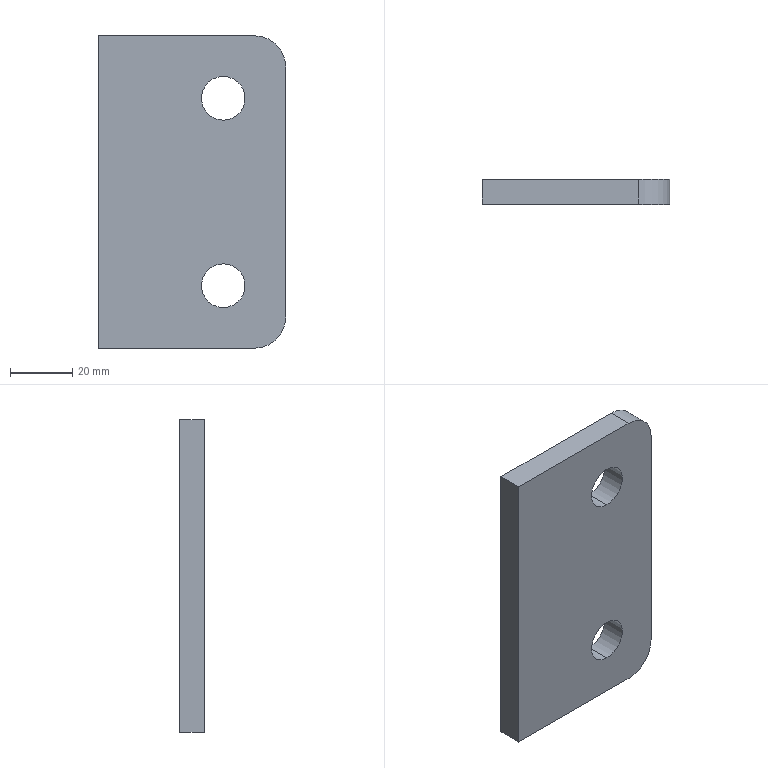Part | SolidWorks | features Extrusion 1 | 1 solid | 12 faces | box 60 x 8 x 100 mm | volume 45194 mm3 | cylinder 6 | plane 6 | commonest cylinder face diameters 14 x4 20 x2
STEP:
#1=CARTESIAN_POINT('',(10.,8.,23.));
#2=VERTEX_POINT('',#1);
#3=CARTESIAN_POINT('',(10.,8.,37.));
#4=VERTEX_POINT('',#3);
#5=CARTESIAN_POINT('',(10.,8.,30.));
#6=DIRECTION('',(0.,1.,0.));
#7=DIRECTION('',(0.,0.,-1.));
#8=AXIS2_PLACEMENT_3D('',#5,#6,#7);
#9=CIRCLE('',#8,7.);
#10=EDGE_CURVE('',#2,#4,#9,.T.);
#11=ORIENTED_EDGE('',*,*,#10,.T.);
#12=CARTESIAN_POINT('',(10.,0.,37.));
#13=VERTEX_POINT('',#12);
#14=CARTESIAN_POINT('',(10.,8.,37.));
#15=DIRECTION('',(0.,-1.,0.));
#16=VECTOR('',#15,1000.);
#17=LINE('',#14,#16);
#18=EDGE_CURVE('',#4,#13,#17,.T.);
#19=ORIENTED_EDGE('',*,*,#18,.T.);
#20=CARTESIAN_POINT('',(10.,0.,23.));
#21=VERTEX_POINT('',#20);
#22=CARTESIAN_POINT('',(10.,0.,30.));
#23=DIRECTION('',(0.,1.,0.));
#24=DIRECTION('',(0.,0.,-1.));
#25=AXIS2_PLACEMENT_3D('',#22,#23,#24);
#26=CIRCLE('',#25,7.);
#27=EDGE_CURVE('',#21,#13,#26,.T.);
#28=ORIENTED_EDGE('',*,*,#27,.F.);
#29=CARTESIAN_POINT('',(10.,8.,23.));
#30=DIRECTION('',(0.,-1.,0.));
#31=VECTOR('',#30,1000.);
#32=LINE('',#29,#31);
#33=EDGE_CURVE('',#2,#21,#32,.T.);
#34=ORIENTED_EDGE('',*,*,#33,.F.);
#35=EDGE_LOOP('',(#11,#19,#28,#34));
#36=FACE_OUTER_BOUND('',#35,.T.);
#37=CARTESIAN_POINT('',(10.,8.,30.));
#38=DIRECTION('',(0.,-1.,0.));
#39=DIRECTION('',(0.,0.,-1.));
#40=AXIS2_PLACEMENT_3D('',#37,#38,#39);
#41=CYLINDRICAL_SURFACE('',#40,7.);
#42=ADVANCED_FACE('',(#36),#41,.F.);
#43=CARTESIAN_POINT('',(10.,8.,-37.));
#44=VERTEX_POINT('',#43);
#45=CARTESIAN_POINT('',(10.,8.,-23.));
#46=VERTEX_POINT('',#45);
#47=CARTESIAN_POINT('',(10.,8.,-30.));
#48=DIRECTION('',(0.,1.,0.));
#49=DIRECTION('',(0.,0.,1.));
#50=AXIS2_PLACEMENT_3D('',#47,#48,#49);
#51=CIRCLE('',#50,7.);
#52=EDGE_CURVE('',#44,#46,#51,.T.);
#53=ORIENTED_EDGE('',*,*,#52,.T.);
#54=CARTESIAN_POINT('',(10.,0.,-23.));
#55=VERTEX_POINT('',#54);
#56=CARTESIAN_POINT('',(10.,8.,-23.));
#57=DIRECTION('',(0.,-1.,0.));
#58=VECTOR('',#57,1000.);
#59=LINE('',#56,#58);
#60=EDGE_CURVE('',#46,#55,#59,.T.);
#61=ORIENTED_EDGE('',*,*,#60,.T.);
#62=CARTESIAN_POINT('',(10.,0.,-37.));
#63=VERTEX_POINT('',#62);
#64=CARTESIAN_POINT('',(10.,0.,-30.));
#65=DIRECTION('',(0.,1.,0.));
#66=DIRECTION('',(0.,0.,1.));
#67=AXIS2_PLACEMENT_3D('',#64,#65,#66);
#68=CIRCLE('',#67,7.);
#69=EDGE_CURVE('',#63,#55,#68,.T.);
#70=ORIENTED_EDGE('',*,*,#69,.F.);
#71=CARTESIAN_POINT('',(10.,8.,-37.));
#72=DIRECTION('',(0.,-1.,0.));
#73=VECTOR('',#72,1000.);
#74=LINE('',#71,#73);
#75=EDGE_CURVE('',#44,#63,#74,.T.);
#76=ORIENTED_EDGE('',*,*,#75,.F.);
#77=EDGE_LOOP('',(#53,#61,#70,#76));
#78=FACE_OUTER_BOUND('',#77,.T.);
#79=CARTESIAN_POINT('',(10.,8.,-30.));
#80=DIRECTION('',(0.,-1.,0.));
#81=DIRECTION('',(0.,0.,-1.));
#82=AXIS2_PLACEMENT_3D('',#79,#80,#81);
#83=CYLINDRICAL_SURFACE('',#82,7.);
#84=ADVANCED_FACE('',(#78),#83,.F.);
#85=CARTESIAN_POINT('',(-30.,8.,-50.));
#86=VERTEX_POINT('',#85);
#87=CARTESIAN_POINT('',(-30.,8.,50.));
#88=VERTEX_POINT('',#87);
#89=CARTESIAN_POINT('',(-30.,8.,50.));
#90=DIRECTION('',(0.,0.,1.));
#91=VECTOR('',#90,1000.);
#92=LINE('',#89,#91);
#93=EDGE_CURVE('',#86,#88,#92,.T.);
#94=ORIENTED_EDGE('',*,*,#93,.T.);
#95=CARTESIAN_POINT('',(20.,8.,50.));
#96=VERTEX_POINT('',#95);
#97=CARTESIAN_POINT('',(-30.,8.,50.));
#98=DIRECTION('',(1.,0.,0.));
#99=VECTOR('',#98,1000.);
#100=LINE('',#97,#99);
#101=EDGE_CURVE('',#88,#96,#100,.T.);
#102=ORIENTED_EDGE('',*,*,#101,.T.);
#103=CARTESIAN_POINT('',(30.,8.,40.));
#104=VERTEX_POINT('',#103);
#105=CARTESIAN_POINT('',(20.,8.,40.));
#106=DIRECTION('',(0.,1.,0.));
#107=DIRECTION('',(0.,0.,1.));
#108=AXIS2_PLACEMENT_3D('',#105,#106,#107);
#109=CIRCLE('',#108,10.);
#110=EDGE_CURVE('',#96,#104,#109,.T.);
#111=ORIENTED_EDGE('',*,*,#110,.T.);
#112=CARTESIAN_POINT('',(30.,8.,-40.));
#113=VERTEX_POINT('',#112);
#114=CARTESIAN_POINT('',(30.,8.,40.));
#115=DIRECTION('',(0.,0.,-1.));
#116=VECTOR('',#115,1000.);
#117=LINE('',#114,#116);
#118=EDGE_CURVE('',#104,#113,#117,.T.);
#119=ORIENTED_EDGE('',*,*,#118,.T.);
#120=CARTESIAN_POINT('',(20.,8.,-50.));
#121=VERTEX_POINT('',#120);
#122=CARTESIAN_POINT('',(20.,8.,-40.));
#123=DIRECTION('',(0.,1.,0.));
#124=DIRECTION('',(0.,0.,-1.));
#125=AXIS2_PLACEMENT_3D('',#122,#123,#124);
#126=CIRCLE('',#125,10.);
#127=EDGE_CURVE('',#113,#121,#126,.T.);
#128=ORIENTED_EDGE('',*,*,#127,.T.);
#129=CARTESIAN_POINT('',(-30.,8.,-50.));
#130=DIRECTION('',(-1.,0.,0.));
#131=VECTOR('',#130,1000.);
#132=LINE('',#129,#131);
#133=EDGE_CURVE('',#121,#86,#132,.T.);
#134=ORIENTED_EDGE('',*,*,#133,.T.);
#135=EDGE_LOOP('',(#94,#102,#111,#119,#128,#134));
#136=FACE_OUTER_BOUND('',#135,.T.);
#137=ORIENTED_EDGE('',*,*,#52,.F.);
#138=CARTESIAN_POINT('',(10.,8.,-30.));
#139=DIRECTION('',(0.,1.,0.));
#140=DIRECTION('',(0.,0.,1.));
#141=AXIS2_PLACEMENT_3D('',#138,#139,#140);
#142=CIRCLE('',#141,7.);
#143=EDGE_CURVE('',#46,#44,#142,.T.);
#144=ORIENTED_EDGE('',*,*,#143,.F.);
#145=EDGE_LOOP('',(#137,#144));
#146=FACE_BOUND('',#145,.T.);
#147=ORIENTED_EDGE('',*,*,#10,.F.);
#148=CARTESIAN_POINT('',(10.,8.,30.));
#149=DIRECTION('',(0.,1.,0.));
#150=DIRECTION('',(0.,0.,-1.));
#151=AXIS2_PLACEMENT_3D('',#148,#149,#150);
#152=CIRCLE('',#151,7.);
#153=EDGE_CURVE('',#4,#2,#152,.T.);
#154=ORIENTED_EDGE('',*,*,#153,.F.);
#155=EDGE_LOOP('',(#147,#154));
#156=FACE_BOUND('',#155,.T.);
#157=CARTESIAN_POINT('',(20.,8.,-40.));
#158=DIRECTION('',(0.,-1.,0.));
#159=DIRECTION('',(0.,0.,-1.));
#160=AXIS2_PLACEMENT_3D('',#157,#158,#159);
#161=PLANE('',#160);
#162=ADVANCED_FACE('',(#136,#146,#156),#161,.F.);
#163=ORIENTED_EDGE('',*,*,#69,.T.);
#164=CARTESIAN_POINT('',(10.,0.,-30.));
#165=DIRECTION('',(0.,1.,0.));
#166=DIRECTION('',(0.,0.,1.));
#167=AXIS2_PLACEMENT_3D('',#164,#165,#166);
#168=CIRCLE('',#167,7.);
#169=EDGE_CURVE('',#55,#63,#168,.T.);
#170=ORIENTED_EDGE('',*,*,#169,.T.);
#171=EDGE_LOOP('',(#163,#170));
#172=FACE_BOUND('',#171,.T.);
#173=CARTESIAN_POINT('',(-30.,0.,-50.));
#174=VERTEX_POINT('',#173);
#175=CARTESIAN_POINT('',(-30.,0.,50.));
#176=VERTEX_POINT('',#175);
#177=CARTESIAN_POINT('',(-30.,0.,50.));
#178=DIRECTION('',(0.,0.,1.));
#179=VECTOR('',#178,1000.);
#180=LINE('',#177,#179);
#181=EDGE_CURVE('',#174,#176,#180,.T.);
#182=ORIENTED_EDGE('',*,*,#181,.F.);
#183=CARTESIAN_POINT('',(20.,0.,-50.));
#184=VERTEX_POINT('',#183);
#185=CARTESIAN_POINT('',(-30.,0.,-50.));
#186=DIRECTION('',(-1.,0.,0.));
#187=VECTOR('',#186,1000.);
#188=LINE('',#185,#187);
#189=EDGE_CURVE('',#184,#174,#188,.T.);
#190=ORIENTED_EDGE('',*,*,#189,.F.);
#191=CARTESIAN_POINT('',(30.,0.,-40.));
#192=VERTEX_POINT('',#191);
#193=CARTESIAN_POINT('',(20.,0.,-40.));
#194=DIRECTION('',(0.,1.,0.));
#195=DIRECTION('',(0.,0.,-1.));
#196=AXIS2_PLACEMENT_3D('',#193,#194,#195);
#197=CIRCLE('',#196,10.);
#198=EDGE_CURVE('',#192,#184,#197,.T.);
#199=ORIENTED_EDGE('',*,*,#198,.F.);
#200=CARTESIAN_POINT('',(30.,0.,40.));
#201=VERTEX_POINT('',#200);
#202=CARTESIAN_POINT('',(30.,0.,40.));
#203=DIRECTION('',(0.,0.,-1.));
#204=VECTOR('',#203,1000.);
#205=LINE('',#202,#204);
#206=EDGE_CURVE('',#201,#192,#205,.T.);
#207=ORIENTED_EDGE('',*,*,#206,.F.);
#208=CARTESIAN_POINT('',(20.,0.,50.));
#209=VERTEX_POINT('',#208);
#210=CARTESIAN_POINT('',(20.,0.,40.));
#211=DIRECTION('',(0.,1.,0.));
#212=DIRECTION('',(0.,0.,1.));
#213=AXIS2_PLACEMENT_3D('',#210,#211,#212);
#214=CIRCLE('',#213,10.);
#215=EDGE_CURVE('',#209,#201,#214,.T.);
#216=ORIENTED_EDGE('',*,*,#215,.F.);
#217=CARTESIAN_POINT('',(-30.,0.,50.));
#218=DIRECTION('',(1.,0.,0.));
#219=VECTOR('',#218,1000.);
#220=LINE('',#217,#219);
#221=EDGE_CURVE('',#176,#209,#220,.T.);
#222=ORIENTED_EDGE('',*,*,#221,.F.);
#223=EDGE_LOOP('',(#182,#190,#199,#207,#216,#222));
#224=FACE_OUTER_BOUND('',#223,.T.);
#225=ORIENTED_EDGE('',*,*,#27,.T.);
#226=CARTESIAN_POINT('',(10.,0.,30.));
#227=DIRECTION('',(0.,1.,0.));
#228=DIRECTION('',(0.,0.,-1.));
#229=AXIS2_PLACEMENT_3D('',#226,#227,#228);
#230=CIRCLE('',#229,7.);
#231=EDGE_CURVE('',#13,#21,#230,.T.);
#232=ORIENTED_EDGE('',*,*,#231,.T.);
#233=EDGE_LOOP('',(#225,#232));
#234=FACE_BOUND('',#233,.T.);
#235=CARTESIAN_POINT('',(20.,0.,-40.));
#236=DIRECTION('',(0.,-1.,0.));
#237=DIRECTION('',(0.,0.,-1.));
#238=AXIS2_PLACEMENT_3D('',#235,#236,#237);
#239=PLANE('',#238);
#240=ADVANCED_FACE('',(#172,#224,#234),#239,.T.);
#241=ORIENTED_EDGE('',*,*,#181,.T.);
#242=CARTESIAN_POINT('',(-30.,8.,50.));
#243=DIRECTION('',(0.,-1.,0.));
#244=VECTOR('',#243,1000.);
#245=LINE('',#242,#244);
#246=EDGE_CURVE('',#88,#176,#245,.T.);
#247=ORIENTED_EDGE('',*,*,#246,.F.);
#248=ORIENTED_EDGE('',*,*,#93,.F.);
#249=CARTESIAN_POINT('',(-30.,8.,-50.));
#250=DIRECTION('',(0.,-1.,0.));
#251=VECTOR('',#250,1000.);
#252=LINE('',#249,#251);
#253=EDGE_CURVE('',#86,#174,#252,.T.);
#254=ORIENTED_EDGE('',*,*,#253,.T.);
#255=EDGE_LOOP('',(#241,#247,#248,#254));
#256=FACE_OUTER_BOUND('',#255,.T.);
#257=CARTESIAN_POINT('',(-30.,8.,50.));
#258=DIRECTION('',(1.,0.,0.));
#259=DIRECTION('',(0.,0.,-1.));
#260=AXIS2_PLACEMENT_3D('',#257,#258,#259);
#261=PLANE('',#260);
#262=ADVANCED_FACE('',(#256),#261,.F.);
#263=ORIENTED_EDGE('',*,*,#221,.T.);
#264=CARTESIAN_POINT('',(20.,8.,50.));
#265=DIRECTION('',(0.,-1.,0.));
#266=VECTOR('',#265,1000.);
#267=LINE('',#264,#266);
#268=EDGE_CURVE('',#96,#209,#267,.T.);
#269=ORIENTED_EDGE('',*,*,#268,.F.);
#270=ORIENTED_EDGE('',*,*,#101,.F.);
#271=ORIENTED_EDGE('',*,*,#246,.T.);
#272=EDGE_LOOP('',(#263,#269,#270,#271));
#273=FACE_OUTER_BOUND('',#272,.T.);
#274=CARTESIAN_POINT('',(-30.,8.,50.));
#275=DIRECTION('',(0.,0.,-1.));
#276=DIRECTION('',(-1.,0.,0.));
#277=AXIS2_PLACEMENT_3D('',#274,#275,#276);
#278=PLANE('',#277);
#279=ADVANCED_FACE('',(#273),#278,.F.);
#280=ORIENTED_EDGE('',*,*,#215,.T.);
#281=CARTESIAN_POINT('',(30.,8.,40.));
#282=DIRECTION('',(0.,-1.,0.));
#283=VECTOR('',#282,1000.);
#284=LINE('',#281,#283);
#285=EDGE_CURVE('',#104,#201,#284,.T.);
#286=ORIENTED_EDGE('',*,*,#285,.F.);
#287=ORIENTED_EDGE('',*,*,#110,.F.);
#288=ORIENTED_EDGE('',*,*,#268,.T.);
#289=EDGE_LOOP('',(#280,#286,#287,#288));
#290=FACE_OUTER_BOUND('',#289,.T.);
#291=CARTESIAN_POINT('',(20.,8.,40.));
#292=DIRECTION('',(0.,-1.,0.));
#293=DIRECTION('',(0.,0.,-1.));
#294=AXIS2_PLACEMENT_3D('',#291,#292,#293);
#295=CYLINDRICAL_SURFACE('',#294,10.);
#296=ADVANCED_FACE('',(#290),#295,.T.);
#297=ORIENTED_EDGE('',*,*,#206,.T.);
#298=CARTESIAN_POINT('',(30.,8.,-40.));
#299=DIRECTION('',(0.,-1.,0.));
#300=VECTOR('',#299,1000.);
#301=LINE('',#298,#300);
#302=EDGE_CURVE('',#113,#192,#301,.T.);
#303=ORIENTED_EDGE('',*,*,#302,.F.);
#304=ORIENTED_EDGE('',*,*,#118,.F.);
#305=ORIENTED_EDGE('',*,*,#285,.T.);
#306=EDGE_LOOP('',(#297,#303,#304,#305));
#307=FACE_OUTER_BOUND('',#306,.T.);
#308=CARTESIAN_POINT('',(30.,8.,40.));
#309=DIRECTION('',(-1.,0.,0.));
#310=DIRECTION('',(0.,0.,1.));
#311=AXIS2_PLACEMENT_3D('',#308,#309,#310);
#312=PLANE('',#311);
#313=ADVANCED_FACE('',(#307),#312,.F.);
#314=ORIENTED_EDGE('',*,*,#198,.T.);
#315=CARTESIAN_POINT('',(20.,8.,-50.));
#316=DIRECTION('',(0.,-1.,0.));
#317=VECTOR('',#316,1000.);
#318=LINE('',#315,#317);
#319=EDGE_CURVE('',#121,#184,#318,.T.);
#320=ORIENTED_EDGE('',*,*,#319,.F.);
#321=ORIENTED_EDGE('',*,*,#127,.F.);
#322=ORIENTED_EDGE('',*,*,#302,.T.);
#323=EDGE_LOOP('',(#314,#320,#321,#322));
#324=FACE_OUTER_BOUND('',#323,.T.);
#325=CARTESIAN_POINT('',(20.,8.,-40.));
#326=DIRECTION('',(0.,-1.,0.));
#327=DIRECTION('',(0.,0.,-1.));
#328=AXIS2_PLACEMENT_3D('',#325,#326,#327);
#329=CYLINDRICAL_SURFACE('',#328,10.);
#330=ADVANCED_FACE('',(#324),#329,.T.);
#331=ORIENTED_EDGE('',*,*,#189,.T.);
#332=ORIENTED_EDGE('',*,*,#253,.F.);
#333=ORIENTED_EDGE('',*,*,#133,.F.);
#334=ORIENTED_EDGE('',*,*,#319,.T.);
#335=EDGE_LOOP('',(#331,#332,#333,#334));
#336=FACE_OUTER_BOUND('',#335,.T.);
#337=CARTESIAN_POINT('',(-30.,8.,-50.));
#338=DIRECTION('',(0.,0.,1.));
#339=DIRECTION('',(1.,0.,0.));
#340=AXIS2_PLACEMENT_3D('',#337,#338,#339);
#341=PLANE('',#340);
#342=ADVANCED_FACE('',(#336),#341,.F.);
#343=ORIENTED_EDGE('',*,*,#60,.F.);
#344=ORIENTED_EDGE('',*,*,#143,.T.);
#345=ORIENTED_EDGE('',*,*,#75,.T.);
#346=ORIENTED_EDGE('',*,*,#169,.F.);
#347=EDGE_LOOP('',(#343,#344,#345,#346));
#348=FACE_OUTER_BOUND('',#347,.T.);
#349=CARTESIAN_POINT('',(10.,8.,-30.));
#350=DIRECTION('',(0.,-1.,0.));
#351=DIRECTION('',(0.,0.,-1.));
#352=AXIS2_PLACEMENT_3D('',#349,#350,#351);
#353=CYLINDRICAL_SURFACE('',#352,7.);
#354=ADVANCED_FACE('',(#348),#353,.F.);
#355=ORIENTED_EDGE('',*,*,#18,.F.);
#356=ORIENTED_EDGE('',*,*,#153,.T.);
#357=ORIENTED_EDGE('',*,*,#33,.T.);
#358=ORIENTED_EDGE('',*,*,#231,.F.);
#359=EDGE_LOOP('',(#355,#356,#357,#358));
#360=FACE_OUTER_BOUND('',#359,.T.);
#361=CARTESIAN_POINT('',(10.,8.,30.));
#362=DIRECTION('',(0.,-1.,0.));
#363=DIRECTION('',(0.,0.,-1.));
#364=AXIS2_PLACEMENT_3D('',#361,#362,#363);
#365=CYLINDRICAL_SURFACE('',#364,7.);
#366=ADVANCED_FACE('',(#360),#365,.F.);
#367=CLOSED_SHELL('',(#42,#84,#162,#240,#262,#279,#296,#313,#330,#342,#354,#366));
#368=MANIFOLD_SOLID_BREP('',#367);
#369=CARTESIAN_POINT('',(0.,0.,0.));
#370=DIRECTION('',(0.,0.,1.));
#371=DIRECTION('',(1.,0.,0.));
#372=AXIS2_PLACEMENT_3D('',#369,#370,#371);
#373=(LENGTH_UNIT()NAMED_UNIT(*)SI_UNIT(.MILLI.,.METRE.));
#374=UNCERTAINTY_MEASURE_WITH_UNIT(LENGTH_MEASURE(0.00001),#373,'','');
#375=(NAMED_UNIT(*)PLANE_ANGLE_UNIT()SI_UNIT($,.RADIAN.));
#376=(NAMED_UNIT(*)SI_UNIT($,.STERADIAN.)SOLID_ANGLE_UNIT());
#377=(GEOMETRIC_REPRESENTATION_CONTEXT(3)GLOBAL_UNCERTAINTY_ASSIGNED_CONTEXT((#374))GLOBAL_UNIT_ASSIGNED_CONTEXT((#373,#375,#376))REPRESENTATION_CONTEXT('',''));
#378=ADVANCED_BREP_SHAPE_REPRESENTATION('',(#368,#372),#377);